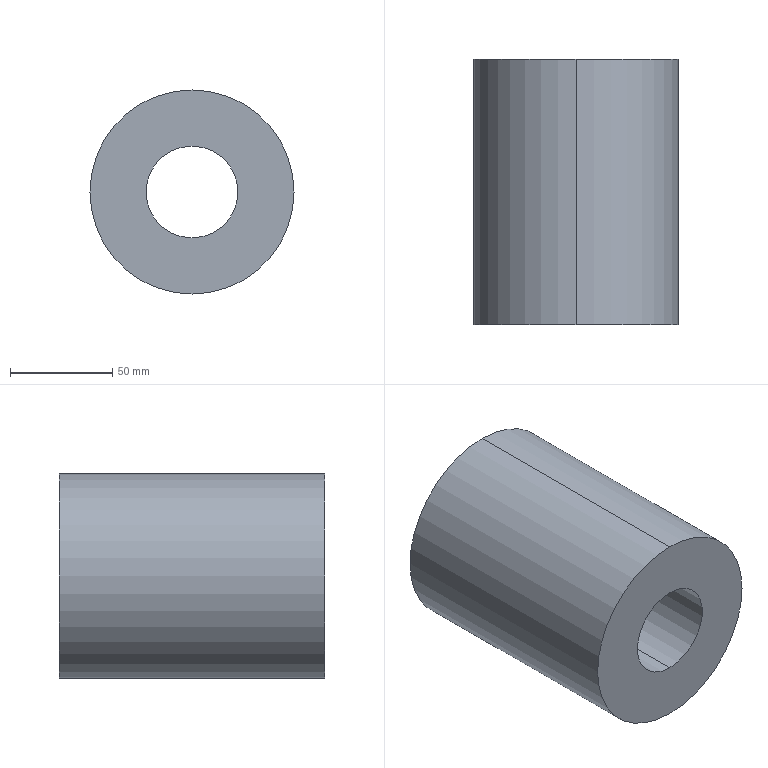Part | SolidWorks | features Extrusion 1 | 1 solid | 6 faces | box 100 x 130 x 100 mm | volume 814262 mm3 | cylinder 4 | plane 2 | commonest cylinder face diameters 45 x2 100 x2
STEP:
#1=CARTESIAN_POINT('',(0.,130.,-22.5));
#2=VERTEX_POINT('',#1);
#3=CARTESIAN_POINT('',(0.,130.,22.5));
#4=VERTEX_POINT('',#3);
#5=CARTESIAN_POINT('',(0.,130.,0.));
#6=DIRECTION('',(0.,1.,0.));
#7=DIRECTION('',(0.,0.,1.));
#8=AXIS2_PLACEMENT_3D('',#5,#6,#7);
#9=CIRCLE('',#8,22.5);
#10=EDGE_CURVE('',#2,#4,#9,.T.);
#11=ORIENTED_EDGE('',*,*,#10,.T.);
#12=CARTESIAN_POINT('',(0.,0.,22.5));
#13=VERTEX_POINT('',#12);
#14=CARTESIAN_POINT('',(0.,130.,22.5));
#15=DIRECTION('',(0.,-1.,0.));
#16=VECTOR('',#15,1000.);
#17=LINE('',#14,#16);
#18=EDGE_CURVE('',#4,#13,#17,.T.);
#19=ORIENTED_EDGE('',*,*,#18,.T.);
#20=CARTESIAN_POINT('',(0.,0.,-22.5));
#21=VERTEX_POINT('',#20);
#22=CARTESIAN_POINT('',(0.,0.,0.));
#23=DIRECTION('',(0.,1.,0.));
#24=DIRECTION('',(0.,0.,1.));
#25=AXIS2_PLACEMENT_3D('',#22,#23,#24);
#26=CIRCLE('',#25,22.5);
#27=EDGE_CURVE('',#21,#13,#26,.T.);
#28=ORIENTED_EDGE('',*,*,#27,.F.);
#29=CARTESIAN_POINT('',(0.,130.,-22.5));
#30=DIRECTION('',(0.,-1.,0.));
#31=VECTOR('',#30,1000.);
#32=LINE('',#29,#31);
#33=EDGE_CURVE('',#2,#21,#32,.T.);
#34=ORIENTED_EDGE('',*,*,#33,.F.);
#35=EDGE_LOOP('',(#11,#19,#28,#34));
#36=FACE_OUTER_BOUND('',#35,.T.);
#37=CARTESIAN_POINT('',(0.,130.,0.));
#38=DIRECTION('',(0.,-1.,0.));
#39=DIRECTION('',(0.,0.,-1.));
#40=AXIS2_PLACEMENT_3D('',#37,#38,#39);
#41=CYLINDRICAL_SURFACE('',#40,22.5);
#42=ADVANCED_FACE('',(#36),#41,.F.);
#43=CARTESIAN_POINT('',(0.,130.,50.));
#44=VERTEX_POINT('',#43);
#45=CARTESIAN_POINT('',(0.,130.,-50.));
#46=VERTEX_POINT('',#45);
#47=CARTESIAN_POINT('',(0.,130.,0.));
#48=DIRECTION('',(0.,1.,0.));
#49=DIRECTION('',(0.,0.,1.));
#50=AXIS2_PLACEMENT_3D('',#47,#48,#49);
#51=CIRCLE('',#50,50.);
#52=EDGE_CURVE('',#44,#46,#51,.T.);
#53=ORIENTED_EDGE('',*,*,#52,.F.);
#54=CARTESIAN_POINT('',(0.,0.,50.));
#55=VERTEX_POINT('',#54);
#56=CARTESIAN_POINT('',(0.,130.,50.));
#57=DIRECTION('',(0.,-1.,0.));
#58=VECTOR('',#57,1000.);
#59=LINE('',#56,#58);
#60=EDGE_CURVE('',#44,#55,#59,.T.);
#61=ORIENTED_EDGE('',*,*,#60,.T.);
#62=CARTESIAN_POINT('',(0.,0.,-50.));
#63=VERTEX_POINT('',#62);
#64=CARTESIAN_POINT('',(0.,0.,0.));
#65=DIRECTION('',(0.,1.,0.));
#66=DIRECTION('',(0.,0.,1.));
#67=AXIS2_PLACEMENT_3D('',#64,#65,#66);
#68=CIRCLE('',#67,50.);
#69=EDGE_CURVE('',#55,#63,#68,.T.);
#70=ORIENTED_EDGE('',*,*,#69,.T.);
#71=CARTESIAN_POINT('',(0.,130.,-50.));
#72=DIRECTION('',(0.,-1.,0.));
#73=VECTOR('',#72,1000.);
#74=LINE('',#71,#73);
#75=EDGE_CURVE('',#46,#63,#74,.T.);
#76=ORIENTED_EDGE('',*,*,#75,.F.);
#77=EDGE_LOOP('',(#53,#61,#70,#76));
#78=FACE_OUTER_BOUND('',#77,.T.);
#79=CARTESIAN_POINT('',(0.,130.,0.));
#80=DIRECTION('',(0.,-1.,0.));
#81=DIRECTION('',(0.,0.,-1.));
#82=AXIS2_PLACEMENT_3D('',#79,#80,#81);
#83=CYLINDRICAL_SURFACE('',#82,50.);
#84=ADVANCED_FACE('',(#78),#83,.T.);
#85=CARTESIAN_POINT('',(0.,130.,0.));
#86=DIRECTION('',(0.,1.,0.));
#87=DIRECTION('',(0.,0.,1.));
#88=AXIS2_PLACEMENT_3D('',#85,#86,#87);
#89=CIRCLE('',#88,50.);
#90=EDGE_CURVE('',#46,#44,#89,.T.);
#91=ORIENTED_EDGE('',*,*,#90,.T.);
#92=ORIENTED_EDGE('',*,*,#52,.T.);
#93=EDGE_LOOP('',(#91,#92));
#94=FACE_OUTER_BOUND('',#93,.T.);
#95=ORIENTED_EDGE('',*,*,#10,.F.);
#96=CARTESIAN_POINT('',(0.,130.,0.));
#97=DIRECTION('',(0.,1.,0.));
#98=DIRECTION('',(0.,0.,1.));
#99=AXIS2_PLACEMENT_3D('',#96,#97,#98);
#100=CIRCLE('',#99,22.5);
#101=EDGE_CURVE('',#4,#2,#100,.T.);
#102=ORIENTED_EDGE('',*,*,#101,.F.);
#103=EDGE_LOOP('',(#95,#102));
#104=FACE_BOUND('',#103,.T.);
#105=CARTESIAN_POINT('',(0.,130.,0.));
#106=DIRECTION('',(0.,1.,0.));
#107=DIRECTION('',(0.,0.,1.));
#108=AXIS2_PLACEMENT_3D('',#105,#106,#107);
#109=PLANE('',#108);
#110=ADVANCED_FACE('',(#94,#104),#109,.T.);
#111=CARTESIAN_POINT('',(0.,0.,0.));
#112=DIRECTION('',(0.,1.,0.));
#113=DIRECTION('',(0.,0.,1.));
#114=AXIS2_PLACEMENT_3D('',#111,#112,#113);
#115=CIRCLE('',#114,50.);
#116=EDGE_CURVE('',#63,#55,#115,.T.);
#117=ORIENTED_EDGE('',*,*,#116,.F.);
#118=ORIENTED_EDGE('',*,*,#69,.F.);
#119=EDGE_LOOP('',(#117,#118));
#120=FACE_OUTER_BOUND('',#119,.T.);
#121=ORIENTED_EDGE('',*,*,#27,.T.);
#122=CARTESIAN_POINT('',(0.,0.,0.));
#123=DIRECTION('',(0.,1.,0.));
#124=DIRECTION('',(0.,0.,1.));
#125=AXIS2_PLACEMENT_3D('',#122,#123,#124);
#126=CIRCLE('',#125,22.5);
#127=EDGE_CURVE('',#13,#21,#126,.T.);
#128=ORIENTED_EDGE('',*,*,#127,.T.);
#129=EDGE_LOOP('',(#121,#128));
#130=FACE_BOUND('',#129,.T.);
#131=CARTESIAN_POINT('',(0.,0.,0.));
#132=DIRECTION('',(0.,1.,0.));
#133=DIRECTION('',(0.,0.,1.));
#134=AXIS2_PLACEMENT_3D('',#131,#132,#133);
#135=PLANE('',#134);
#136=ADVANCED_FACE('',(#120,#130),#135,.F.);
#137=ORIENTED_EDGE('',*,*,#60,.F.);
#138=ORIENTED_EDGE('',*,*,#90,.F.);
#139=ORIENTED_EDGE('',*,*,#75,.T.);
#140=ORIENTED_EDGE('',*,*,#116,.T.);
#141=EDGE_LOOP('',(#137,#138,#139,#140));
#142=FACE_OUTER_BOUND('',#141,.T.);
#143=CARTESIAN_POINT('',(0.,130.,0.));
#144=DIRECTION('',(0.,-1.,0.));
#145=DIRECTION('',(0.,0.,-1.));
#146=AXIS2_PLACEMENT_3D('',#143,#144,#145);
#147=CYLINDRICAL_SURFACE('',#146,50.);
#148=ADVANCED_FACE('',(#142),#147,.T.);
#149=ORIENTED_EDGE('',*,*,#18,.F.);
#150=ORIENTED_EDGE('',*,*,#101,.T.);
#151=ORIENTED_EDGE('',*,*,#33,.T.);
#152=ORIENTED_EDGE('',*,*,#127,.F.);
#153=EDGE_LOOP('',(#149,#150,#151,#152));
#154=FACE_OUTER_BOUND('',#153,.T.);
#155=CARTESIAN_POINT('',(0.,130.,0.));
#156=DIRECTION('',(0.,-1.,0.));
#157=DIRECTION('',(0.,0.,-1.));
#158=AXIS2_PLACEMENT_3D('',#155,#156,#157);
#159=CYLINDRICAL_SURFACE('',#158,22.5);
#160=ADVANCED_FACE('',(#154),#159,.F.);
#161=CLOSED_SHELL('',(#42,#84,#110,#136,#148,#160));
#162=MANIFOLD_SOLID_BREP('',#161);
#163=CARTESIAN_POINT('',(0.,0.,0.));
#164=DIRECTION('',(0.,0.,1.));
#165=DIRECTION('',(1.,0.,0.));
#166=AXIS2_PLACEMENT_3D('',#163,#164,#165);
#167=(LENGTH_UNIT()NAMED_UNIT(*)SI_UNIT(.MILLI.,.METRE.));
#168=UNCERTAINTY_MEASURE_WITH_UNIT(LENGTH_MEASURE(0.00001),#167,'','');
#169=(NAMED_UNIT(*)PLANE_ANGLE_UNIT()SI_UNIT($,.RADIAN.));
#170=(NAMED_UNIT(*)SI_UNIT($,.STERADIAN.)SOLID_ANGLE_UNIT());
#171=(GEOMETRIC_REPRESENTATION_CONTEXT(3)GLOBAL_UNCERTAINTY_ASSIGNED_CONTEXT((#168))GLOBAL_UNIT_ASSIGNED_CONTEXT((#167,#169,#170))REPRESENTATION_CONTEXT('',''));
#172=ADVANCED_BREP_SHAPE_REPRESENTATION('',(#162,#166),#171);